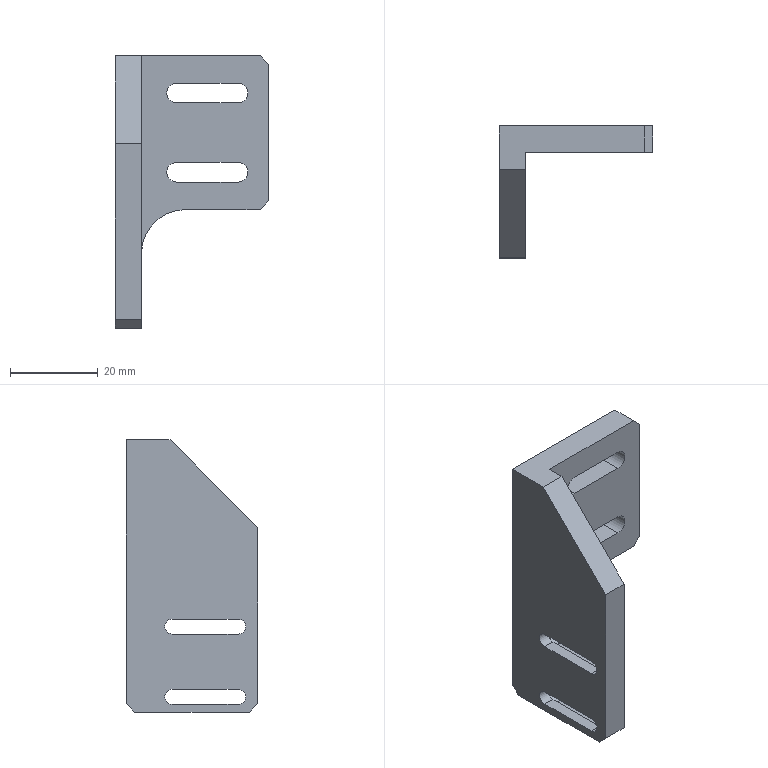Part | STEP file | 0-19 Finger cylinder fixed plate 1 (original) | 1 solid | 41 faces | box 35 x 30 x 62 mm | volume 14067 mm3 | plane 28 | cylinder 13 | commonest cylinder face diameters 3.4 x4 4.5 x4 6 x4 20 x1